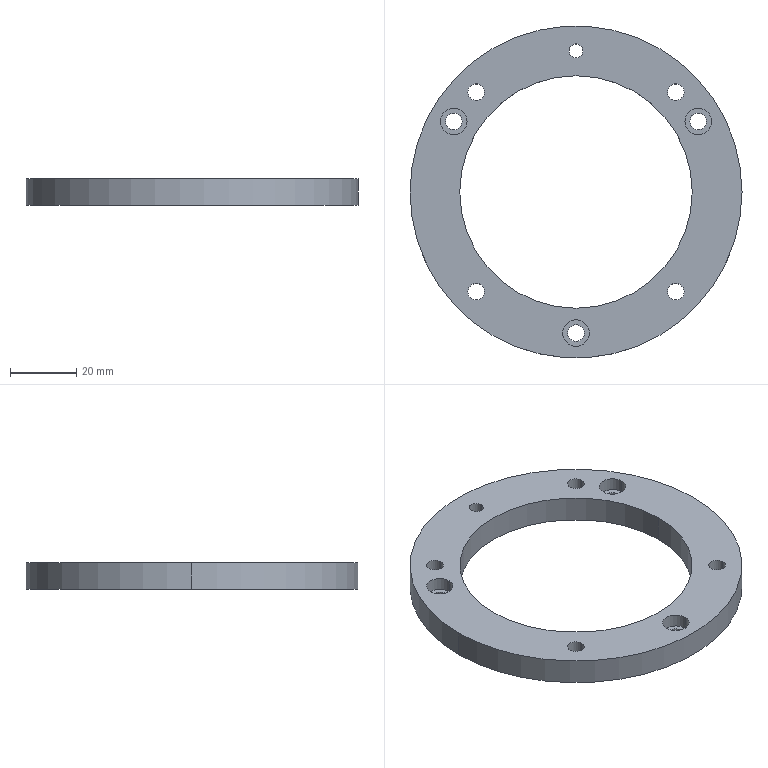Part | SolidWorks | features ICE 5, Extrusion 1 | 1 solid | 31 faces | box 100 x 100 x 8 mm | volume 30466 mm3 | cylinder 26 | plane 5 | commonest cylinder face diameters 5 x14 8 x6 4.2 x2 70 x2 100 x2
STEP:
#1=CARTESIAN_POINT('',(-35.,0.,0.));
#2=VERTEX_POINT('',#1);
#3=CARTESIAN_POINT('',(35.,0.,0.));
#4=VERTEX_POINT('',#3);
#5=CARTESIAN_POINT('',(0.,0.,0.));
#6=DIRECTION('',(0.,0.,1.));
#7=DIRECTION('',(1.,0.,0.));
#8=AXIS2_PLACEMENT_3D('',#5,#6,#7);
#9=CIRCLE('',#8,35.);
#10=EDGE_CURVE('',#2,#4,#9,.T.);
#11=ORIENTED_EDGE('',*,*,#10,.F.);
#12=CARTESIAN_POINT('',(-35.,0.,8.));
#13=VERTEX_POINT('',#12);
#14=CARTESIAN_POINT('',(-35.,0.,-2.));
#15=DIRECTION('',(0.,0.,1.));
#16=VECTOR('',#15,1000.);
#17=LINE('',#14,#16);
#18=EDGE_CURVE('',#2,#13,#17,.T.);
#19=ORIENTED_EDGE('',*,*,#18,.T.);
#20=CARTESIAN_POINT('',(35.,0.,8.));
#21=VERTEX_POINT('',#20);
#22=CARTESIAN_POINT('',(0.,0.,8.));
#23=DIRECTION('',(0.,0.,1.));
#24=DIRECTION('',(1.,0.,0.));
#25=AXIS2_PLACEMENT_3D('',#22,#23,#24);
#26=CIRCLE('',#25,35.);
#27=EDGE_CURVE('',#13,#21,#26,.T.);
#28=ORIENTED_EDGE('',*,*,#27,.T.);
#29=CARTESIAN_POINT('',(35.,0.,-2.));
#30=DIRECTION('',(0.,0.,1.));
#31=VECTOR('',#30,1000.);
#32=LINE('',#29,#31);
#33=EDGE_CURVE('',#4,#21,#32,.T.);
#34=ORIENTED_EDGE('',*,*,#33,.F.);
#35=EDGE_LOOP('',(#11,#19,#28,#34));
#36=FACE_OUTER_BOUND('',#35,.T.);
#37=CARTESIAN_POINT('',(0.,0.,-2.));
#38=DIRECTION('',(0.,0.,1.));
#39=DIRECTION('',(1.,0.,0.));
#40=AXIS2_PLACEMENT_3D('',#37,#38,#39);
#41=CYLINDRICAL_SURFACE('',#40,35.);
#42=ADVANCED_FACE('',(#36),#41,.F.);
#43=CARTESIAN_POINT('',(34.306,21.25,0.));
#44=VERTEX_POINT('',#43);
#45=CARTESIAN_POINT('',(39.306,21.25,0.));
#46=VERTEX_POINT('',#45);
#47=CARTESIAN_POINT('',(36.806,21.25,0.));
#48=DIRECTION('',(0.,0.,1.));
#49=DIRECTION('',(1.,0.,0.));
#50=AXIS2_PLACEMENT_3D('',#47,#48,#49);
#51=CIRCLE('',#50,2.5);
#52=EDGE_CURVE('',#44,#46,#51,.T.);
#53=ORIENTED_EDGE('',*,*,#52,.F.);
#54=CARTESIAN_POINT('',(34.306,21.25,4.));
#55=VERTEX_POINT('',#54);
#56=CARTESIAN_POINT('',(34.306,21.25,0.));
#57=DIRECTION('',(0.,0.,1.));
#58=VECTOR('',#57,1000.);
#59=LINE('',#56,#58);
#60=EDGE_CURVE('',#44,#55,#59,.T.);
#61=ORIENTED_EDGE('',*,*,#60,.T.);
#62=CARTESIAN_POINT('',(39.306,21.25,4.));
#63=VERTEX_POINT('',#62);
#64=CARTESIAN_POINT('',(36.806,21.25,4.));
#65=DIRECTION('',(0.,0.,1.));
#66=DIRECTION('',(1.,0.,0.));
#67=AXIS2_PLACEMENT_3D('',#64,#65,#66);
#68=CIRCLE('',#67,2.5);
#69=EDGE_CURVE('',#55,#63,#68,.T.);
#70=ORIENTED_EDGE('',*,*,#69,.T.);
#71=CARTESIAN_POINT('',(39.306,21.25,0.));
#72=DIRECTION('',(0.,0.,1.));
#73=VECTOR('',#72,1000.);
#74=LINE('',#71,#73);
#75=EDGE_CURVE('',#46,#63,#74,.T.);
#76=ORIENTED_EDGE('',*,*,#75,.F.);
#77=EDGE_LOOP('',(#53,#61,#70,#76));
#78=FACE_OUTER_BOUND('',#77,.T.);
#79=CARTESIAN_POINT('',(36.806,21.25,0.));
#80=DIRECTION('',(0.,0.,1.));
#81=DIRECTION('',(1.,0.,0.));
#82=AXIS2_PLACEMENT_3D('',#79,#80,#81);
#83=CYLINDRICAL_SURFACE('',#82,2.5);
#84=ADVANCED_FACE('',(#78),#83,.F.);
#85=CARTESIAN_POINT('',(-2.5,-42.5,0.));
#86=VERTEX_POINT('',#85);
#87=CARTESIAN_POINT('',(2.5,-42.5,0.));
#88=VERTEX_POINT('',#87);
#89=CARTESIAN_POINT('',(0.,-42.5,0.));
#90=DIRECTION('',(0.,0.,1.));
#91=DIRECTION('',(1.,0.,0.));
#92=AXIS2_PLACEMENT_3D('',#89,#90,#91);
#93=CIRCLE('',#92,2.5);
#94=EDGE_CURVE('',#86,#88,#93,.T.);
#95=ORIENTED_EDGE('',*,*,#94,.F.);
#96=CARTESIAN_POINT('',(-2.5,-42.5,4.));
#97=VERTEX_POINT('',#96);
#98=CARTESIAN_POINT('',(-2.5,-42.5,0.));
#99=DIRECTION('',(0.,0.,1.));
#100=VECTOR('',#99,1000.);
#101=LINE('',#98,#100);
#102=EDGE_CURVE('',#86,#97,#101,.T.);
#103=ORIENTED_EDGE('',*,*,#102,.T.);
#104=CARTESIAN_POINT('',(2.5,-42.5,4.));
#105=VERTEX_POINT('',#104);
#106=CARTESIAN_POINT('',(0.,-42.5,4.));
#107=DIRECTION('',(0.,0.,1.));
#108=DIRECTION('',(1.,0.,0.));
#109=AXIS2_PLACEMENT_3D('',#106,#107,#108);
#110=CIRCLE('',#109,2.5);
#111=EDGE_CURVE('',#97,#105,#110,.T.);
#112=ORIENTED_EDGE('',*,*,#111,.T.);
#113=CARTESIAN_POINT('',(2.5,-42.5,0.));
#114=DIRECTION('',(0.,0.,1.));
#115=VECTOR('',#114,1000.);
#116=LINE('',#113,#115);
#117=EDGE_CURVE('',#88,#105,#116,.T.);
#118=ORIENTED_EDGE('',*,*,#117,.F.);
#119=EDGE_LOOP('',(#95,#103,#112,#118));
#120=FACE_OUTER_BOUND('',#119,.T.);
#121=CARTESIAN_POINT('',(0.,-42.5,0.));
#122=DIRECTION('',(0.,0.,1.));
#123=DIRECTION('',(1.,0.,0.));
#124=AXIS2_PLACEMENT_3D('',#121,#122,#123);
#125=CYLINDRICAL_SURFACE('',#124,2.5);
#126=ADVANCED_FACE('',(#120),#125,.F.);
#127=CARTESIAN_POINT('',(-39.306,21.25,0.));
#128=VERTEX_POINT('',#127);
#129=CARTESIAN_POINT('',(-34.306,21.25,0.));
#130=VERTEX_POINT('',#129);
#131=CARTESIAN_POINT('',(-36.806,21.25,0.));
#132=DIRECTION('',(0.,0.,1.));
#133=DIRECTION('',(1.,0.,0.));
#134=AXIS2_PLACEMENT_3D('',#131,#132,#133);
#135=CIRCLE('',#134,2.5);
#136=EDGE_CURVE('',#128,#130,#135,.T.);
#137=ORIENTED_EDGE('',*,*,#136,.F.);
#138=CARTESIAN_POINT('',(-39.306,21.25,4.));
#139=VERTEX_POINT('',#138);
#140=CARTESIAN_POINT('',(-39.306,21.25,0.));
#141=DIRECTION('',(0.,0.,1.));
#142=VECTOR('',#141,1000.);
#143=LINE('',#140,#142);
#144=EDGE_CURVE('',#128,#139,#143,.T.);
#145=ORIENTED_EDGE('',*,*,#144,.T.);
#146=CARTESIAN_POINT('',(-34.306,21.25,4.));
#147=VERTEX_POINT('',#146);
#148=CARTESIAN_POINT('',(-36.806,21.25,4.));
#149=DIRECTION('',(0.,0.,1.));
#150=DIRECTION('',(1.,0.,0.));
#151=AXIS2_PLACEMENT_3D('',#148,#149,#150);
#152=CIRCLE('',#151,2.5);
#153=EDGE_CURVE('',#139,#147,#152,.T.);
#154=ORIENTED_EDGE('',*,*,#153,.T.);
#155=CARTESIAN_POINT('',(-34.306,21.25,0.));
#156=DIRECTION('',(0.,0.,1.));
#157=VECTOR('',#156,1000.);
#158=LINE('',#155,#157);
#159=EDGE_CURVE('',#130,#147,#158,.T.);
#160=ORIENTED_EDGE('',*,*,#159,.F.);
#161=EDGE_LOOP('',(#137,#145,#154,#160));
#162=FACE_OUTER_BOUND('',#161,.T.);
#163=CARTESIAN_POINT('',(-36.806,21.25,0.));
#164=DIRECTION('',(0.,0.,1.));
#165=DIRECTION('',(1.,0.,0.));
#166=AXIS2_PLACEMENT_3D('',#163,#164,#165);
#167=CYLINDRICAL_SURFACE('',#166,2.5);
#168=ADVANCED_FACE('',(#162),#167,.F.);
#169=CARTESIAN_POINT('',(32.806,21.25,4.));
#170=VERTEX_POINT('',#169);
#171=CARTESIAN_POINT('',(40.806,21.25,4.));
#172=VERTEX_POINT('',#171);
#173=CARTESIAN_POINT('',(36.806,21.25,4.));
#174=DIRECTION('',(0.,0.,1.));
#175=DIRECTION('',(1.,0.,0.));
#176=AXIS2_PLACEMENT_3D('',#173,#174,#175);
#177=CIRCLE('',#176,4.);
#178=EDGE_CURVE('',#170,#172,#177,.T.);
#179=ORIENTED_EDGE('',*,*,#178,.F.);
#180=CARTESIAN_POINT('',(32.806,21.25,8.));
#181=VERTEX_POINT('',#180);
#182=CARTESIAN_POINT('',(32.806,21.25,4.));
#183=DIRECTION('',(0.,0.,1.));
#184=VECTOR('',#183,1000.);
#185=LINE('',#182,#184);
#186=EDGE_CURVE('',#170,#181,#185,.T.);
#187=ORIENTED_EDGE('',*,*,#186,.T.);
#188=CARTESIAN_POINT('',(40.806,21.25,8.));
#189=VERTEX_POINT('',#188);
#190=CARTESIAN_POINT('',(36.806,21.25,8.));
#191=DIRECTION('',(0.,0.,1.));
#192=DIRECTION('',(1.,0.,0.));
#193=AXIS2_PLACEMENT_3D('',#190,#191,#192);
#194=CIRCLE('',#193,4.);
#195=EDGE_CURVE('',#181,#189,#194,.T.);
#196=ORIENTED_EDGE('',*,*,#195,.T.);
#197=CARTESIAN_POINT('',(40.806,21.25,4.));
#198=DIRECTION('',(0.,0.,1.));
#199=VECTOR('',#198,1000.);
#200=LINE('',#197,#199);
#201=EDGE_CURVE('',#172,#189,#200,.T.);
#202=ORIENTED_EDGE('',*,*,#201,.F.);
#203=EDGE_LOOP('',(#179,#187,#196,#202));
#204=FACE_OUTER_BOUND('',#203,.T.);
#205=CARTESIAN_POINT('',(36.806,21.25,4.));
#206=DIRECTION('',(0.,0.,1.));
#207=DIRECTION('',(1.,0.,0.));
#208=AXIS2_PLACEMENT_3D('',#205,#206,#207);
#209=CYLINDRICAL_SURFACE('',#208,4.);
#210=ADVANCED_FACE('',(#204),#209,.F.);
#211=CARTESIAN_POINT('',(-40.806,21.25,4.));
#212=VERTEX_POINT('',#211);
#213=CARTESIAN_POINT('',(-32.806,21.25,4.));
#214=VERTEX_POINT('',#213);
#215=CARTESIAN_POINT('',(-36.806,21.25,4.));
#216=DIRECTION('',(0.,0.,1.));
#217=DIRECTION('',(1.,0.,0.));
#218=AXIS2_PLACEMENT_3D('',#215,#216,#217);
#219=CIRCLE('',#218,4.);
#220=EDGE_CURVE('',#212,#214,#219,.T.);
#221=ORIENTED_EDGE('',*,*,#220,.F.);
#222=CARTESIAN_POINT('',(-40.806,21.25,8.));
#223=VERTEX_POINT('',#222);
#224=CARTESIAN_POINT('',(-40.806,21.25,4.));
#225=DIRECTION('',(0.,0.,1.));
#226=VECTOR('',#225,1000.);
#227=LINE('',#224,#226);
#228=EDGE_CURVE('',#212,#223,#227,.T.);
#229=ORIENTED_EDGE('',*,*,#228,.T.);
#230=CARTESIAN_POINT('',(-32.806,21.25,8.));
#231=VERTEX_POINT('',#230);
#232=CARTESIAN_POINT('',(-36.806,21.25,8.));
#233=DIRECTION('',(0.,0.,1.));
#234=DIRECTION('',(1.,0.,0.));
#235=AXIS2_PLACEMENT_3D('',#232,#233,#234);
#236=CIRCLE('',#235,4.);
#237=EDGE_CURVE('',#223,#231,#236,.T.);
#238=ORIENTED_EDGE('',*,*,#237,.T.);
#239=CARTESIAN_POINT('',(-32.806,21.25,4.));
#240=DIRECTION('',(0.,0.,1.));
#241=VECTOR('',#240,1000.);
#242=LINE('',#239,#241);
#243=EDGE_CURVE('',#214,#231,#242,.T.);
#244=ORIENTED_EDGE('',*,*,#243,.F.);
#245=EDGE_LOOP('',(#221,#229,#238,#244));
#246=FACE_OUTER_BOUND('',#245,.T.);
#247=CARTESIAN_POINT('',(-36.806,21.25,4.));
#248=DIRECTION('',(0.,0.,1.));
#249=DIRECTION('',(1.,0.,0.));
#250=AXIS2_PLACEMENT_3D('',#247,#248,#249);
#251=CYLINDRICAL_SURFACE('',#250,4.);
#252=ADVANCED_FACE('',(#246),#251,.F.);
#253=CARTESIAN_POINT('',(-4.,-42.5,4.));
#254=VERTEX_POINT('',#253);
#255=CARTESIAN_POINT('',(4.,-42.5,4.));
#256=VERTEX_POINT('',#255);
#257=CARTESIAN_POINT('',(0.,-42.5,4.));
#258=DIRECTION('',(0.,0.,1.));
#259=DIRECTION('',(1.,0.,0.));
#260=AXIS2_PLACEMENT_3D('',#257,#258,#259);
#261=CIRCLE('',#260,4.);
#262=EDGE_CURVE('',#254,#256,#261,.T.);
#263=ORIENTED_EDGE('',*,*,#262,.F.);
#264=CARTESIAN_POINT('',(-4.,-42.5,8.));
#265=VERTEX_POINT('',#264);
#266=CARTESIAN_POINT('',(-4.,-42.5,4.));
#267=DIRECTION('',(0.,0.,1.));
#268=VECTOR('',#267,1000.);
#269=LINE('',#266,#268);
#270=EDGE_CURVE('',#254,#265,#269,.T.);
#271=ORIENTED_EDGE('',*,*,#270,.T.);
#272=CARTESIAN_POINT('',(4.,-42.5,8.));
#273=VERTEX_POINT('',#272);
#274=CARTESIAN_POINT('',(0.,-42.5,8.));
#275=DIRECTION('',(0.,0.,1.));
#276=DIRECTION('',(1.,0.,0.));
#277=AXIS2_PLACEMENT_3D('',#274,#275,#276);
#278=CIRCLE('',#277,4.);
#279=EDGE_CURVE('',#265,#273,#278,.T.);
#280=ORIENTED_EDGE('',*,*,#279,.T.);
#281=CARTESIAN_POINT('',(4.,-42.5,4.));
#282=DIRECTION('',(0.,0.,1.));
#283=VECTOR('',#282,1000.);
#284=LINE('',#281,#283);
#285=EDGE_CURVE('',#256,#273,#284,.T.);
#286=ORIENTED_EDGE('',*,*,#285,.F.);
#287=EDGE_LOOP('',(#263,#271,#280,#286));
#288=FACE_OUTER_BOUND('',#287,.T.);
#289=CARTESIAN_POINT('',(0.,-42.5,4.));
#290=DIRECTION('',(0.,0.,1.));
#291=DIRECTION('',(1.,0.,0.));
#292=AXIS2_PLACEMENT_3D('',#289,#290,#291);
#293=CYLINDRICAL_SURFACE('',#292,4.);
#294=ADVANCED_FACE('',(#288),#293,.F.);
#295=CARTESIAN_POINT('',(-2.1,42.5,0.));
#296=VERTEX_POINT('',#295);
#297=CARTESIAN_POINT('',(2.1,42.5,0.));
#298=VERTEX_POINT('',#297);
#299=CARTESIAN_POINT('',(0.,42.5,0.));
#300=DIRECTION('',(0.,0.,1.));
#301=DIRECTION('',(1.,0.,0.));
#302=AXIS2_PLACEMENT_3D('',#299,#300,#301);
#303=CIRCLE('',#302,2.1);
#304=EDGE_CURVE('',#296,#298,#303,.T.);
#305=ORIENTED_EDGE('',*,*,#304,.F.);
#306=CARTESIAN_POINT('',(-2.1,42.5,8.));
#307=VERTEX_POINT('',#306);
#308=CARTESIAN_POINT('',(-2.1,42.5,0.));
#309=DIRECTION('',(0.,0.,1.));
#310=VECTOR('',#309,1000.);
#311=LINE('',#308,#310);
#312=EDGE_CURVE('',#296,#307,#311,.T.);
#313=ORIENTED_EDGE('',*,*,#312,.T.);
#314=CARTESIAN_POINT('',(2.1,42.5,8.));
#315=VERTEX_POINT('',#314);
#316=CARTESIAN_POINT('',(0.,42.5,8.));
#317=DIRECTION('',(0.,0.,1.));
#318=DIRECTION('',(1.,0.,0.));
#319=AXIS2_PLACEMENT_3D('',#316,#317,#318);
#320=CIRCLE('',#319,2.1);
#321=EDGE_CURVE('',#307,#315,#320,.T.);
#322=ORIENTED_EDGE('',*,*,#321,.T.);
#323=CARTESIAN_POINT('',(2.1,42.5,0.));
#324=DIRECTION('',(0.,0.,1.));
#325=VECTOR('',#324,1000.);
#326=LINE('',#323,#325);
#327=EDGE_CURVE('',#298,#315,#326,.T.);
#328=ORIENTED_EDGE('',*,*,#327,.F.);
#329=EDGE_LOOP('',(#305,#313,#322,#328));
#330=FACE_OUTER_BOUND('',#329,.T.);
#331=CARTESIAN_POINT('',(0.,42.5,0.));
#332=DIRECTION('',(0.,0.,1.));
#333=DIRECTION('',(1.,0.,0.));
#334=AXIS2_PLACEMENT_3D('',#331,#332,#333);
#335=CYLINDRICAL_SURFACE('',#334,2.1);
#336=ADVANCED_FACE('',(#330),#335,.F.);
#337=CARTESIAN_POINT('',(27.554,-30.05,0.));
#338=VERTEX_POINT('',#337);
#339=CARTESIAN_POINT('',(32.554,-30.05,0.));
#340=VERTEX_POINT('',#339);
#341=CARTESIAN_POINT('',(30.054,-30.05,0.));
#342=DIRECTION('',(0.,0.,1.));
#343=DIRECTION('',(1.,0.,0.));
#344=AXIS2_PLACEMENT_3D('',#341,#342,#343);
#345=CIRCLE('',#344,2.5);
#346=EDGE_CURVE('',#338,#340,#345,.T.);
#347=ORIENTED_EDGE('',*,*,#346,.F.);
#348=CARTESIAN_POINT('',(27.554,-30.05,8.));
#349=VERTEX_POINT('',#348);
#350=CARTESIAN_POINT('',(27.554,-30.05,0.));
#351=DIRECTION('',(0.,0.,1.));
#352=VECTOR('',#351,1000.);
#353=LINE('',#350,#352);
#354=EDGE_CURVE('',#338,#349,#353,.T.);
#355=ORIENTED_EDGE('',*,*,#354,.T.);
#356=CARTESIAN_POINT('',(32.554,-30.05,8.));
#357=VERTEX_POINT('',#356);
#358=CARTESIAN_POINT('',(30.054,-30.05,8.));
#359=DIRECTION('',(0.,0.,1.));
#360=DIRECTION('',(1.,0.,0.));
#361=AXIS2_PLACEMENT_3D('',#358,#359,#360);
#362=CIRCLE('',#361,2.5);
#363=EDGE_CURVE('',#349,#357,#362,.T.);
#364=ORIENTED_EDGE('',*,*,#363,.T.);
#365=CARTESIAN_POINT('',(32.554,-30.05,0.));
#366=DIRECTION('',(0.,0.,1.));
#367=VECTOR('',#366,1000.);
#368=LINE('',#365,#367);
#369=EDGE_CURVE('',#340,#357,#368,.T.);
#370=ORIENTED_EDGE('',*,*,#369,.F.);
#371=EDGE_LOOP('',(#347,#355,#364,#370));
#372=FACE_OUTER_BOUND('',#371,.T.);
#373=CARTESIAN_POINT('',(30.054,-30.05,0.));
#374=DIRECTION('',(0.,0.,1.));
#375=DIRECTION('',(1.,0.,0.));
#376=AXIS2_PLACEMENT_3D('',#373,#374,#375);
#377=CYLINDRICAL_SURFACE('',#376,2.5);
#378=ADVANCED_FACE('',(#372),#377,.F.);
#379=CARTESIAN_POINT('',(-32.554,-30.05,0.));
#380=VERTEX_POINT('',#379);
#381=CARTESIAN_POINT('',(-27.554,-30.05,0.));
#382=VERTEX_POINT('',#381);
#383=CARTESIAN_POINT('',(-30.054,-30.05,0.));
#384=DIRECTION('',(0.,0.,1.));
#385=DIRECTION('',(1.,0.,0.));
#386=AXIS2_PLACEMENT_3D('',#383,#384,#385);
#387=CIRCLE('',#386,2.5);
#388=EDGE_CURVE('',#380,#382,#387,.T.);
#389=ORIENTED_EDGE('',*,*,#388,.F.);
#390=CARTESIAN_POINT('',(-32.554,-30.05,8.));
#391=VERTEX_POINT('',#390);
#392=CARTESIAN_POINT('',(-32.554,-30.05,0.));
#393=DIRECTION('',(0.,0.,1.));
#394=VECTOR('',#393,1000.);
#395=LINE('',#392,#394);
#396=EDGE_CURVE('',#380,#391,#395,.T.);
#397=ORIENTED_EDGE('',*,*,#396,.T.);
#398=CARTESIAN_POINT('',(-27.554,-30.05,8.));
#399=VERTEX_POINT('',#398);
#400=CARTESIAN_POINT('',(-30.054,-30.05,8.));
#401=DIRECTION('',(0.,0.,1.));
#402=DIRECTION('',(1.,0.,0.));
#403=AXIS2_PLACEMENT_3D('',#400,#401,#402);
#404=CIRCLE('',#403,2.5);
#405=EDGE_CURVE('',#391,#399,#404,.T.);
#406=ORIENTED_EDGE('',*,*,#405,.T.);
#407=CARTESIAN_POINT('',(-27.554,-30.05,0.));
#408=DIRECTION('',(0.,0.,1.));
#409=VECTOR('',#408,1000.);
#410=LINE('',#407,#409);
#411=EDGE_CURVE('',#382,#399,#410,.T.);
#412=ORIENTED_EDGE('',*,*,#411,.F.);
#413=EDGE_LOOP('',(#389,#397,#406,#412));
#414=FACE_OUTER_BOUND('',#413,.T.);
#415=CARTESIAN_POINT('',(-30.054,-30.05,0.));
#416=DIRECTION('',(0.,0.,1.));
#417=DIRECTION('',(1.,0.,0.));
#418=AXIS2_PLACEMENT_3D('',#415,#416,#417);
#419=CYLINDRICAL_SURFACE('',#418,2.5);
#420=ADVANCED_FACE('',(#414),#419,.F.);
#421=CARTESIAN_POINT('',(27.554,30.05,0.));
#422=VERTEX_POINT('',#421);
#423=CARTESIAN_POINT('',(32.554,30.05,0.));
#424=VERTEX_POINT('',#423);
#425=CARTESIAN_POINT('',(30.054,30.05,0.));
#426=DIRECTION('',(0.,0.,1.));
#427=DIRECTION('',(1.,0.,0.));
#428=AXIS2_PLACEMENT_3D('',#425,#426,#427);
#429=CIRCLE('',#428,2.5);
#430=EDGE_CURVE('',#422,#424,#429,.T.);
#431=ORIENTED_EDGE('',*,*,#430,.F.);
#432=CARTESIAN_POINT('',(27.554,30.05,8.));
#433=VERTEX_POINT('',#432);
#434=CARTESIAN_POINT('',(27.554,30.05,0.));
#435=DIRECTION('',(0.,0.,1.));
#436=VECTOR('',#435,1000.);
#437=LINE('',#434,#436);
#438=EDGE_CURVE('',#422,#433,#437,.T.);
#439=ORIENTED_EDGE('',*,*,#438,.T.);
#440=CARTESIAN_POINT('',(32.554,30.05,8.));
#441=VERTEX_POINT('',#440);
#442=CARTESIAN_POINT('',(30.054,30.05,8.));
#443=DIRECTION('',(0.,0.,1.));
#444=DIRECTION('',(1.,0.,0.));
#445=AXIS2_PLACEMENT_3D('',#442,#443,#444);
#446=CIRCLE('',#445,2.5);
#447=EDGE_CURVE('',#433,#441,#446,.T.);
#448=ORIENTED_EDGE('',*,*,#447,.T.);
#449=CARTESIAN_POINT('',(32.554,30.05,0.));
#450=DIRECTION('',(0.,0.,1.));
#451=VECTOR('',#450,1000.);
#452=LINE('',#449,#451);
#453=EDGE_CURVE('',#424,#441,#452,.T.);
#454=ORIENTED_EDGE('',*,*,#453,.F.);
#455=EDGE_LOOP('',(#431,#439,#448,#454));
#456=FACE_OUTER_BOUND('',#455,.T.);
#457=CARTESIAN_POINT('',(30.054,30.05,0.));
#458=DIRECTION('',(0.,0.,1.));
#459=DIRECTION('',(1.,0.,0.));
#460=AXIS2_PLACEMENT_3D('',#457,#458,#459);
#461=CYLINDRICAL_SURFACE('',#460,2.5);
#462=ADVANCED_FACE('',(#456),#461,.F.);
#463=CARTESIAN_POINT('',(-32.554,30.05,0.));
#464=VERTEX_POINT('',#463);
#465=CARTESIAN_POINT('',(-27.554,30.05,0.));
#466=VERTEX_POINT('',#465);
#467=CARTESIAN_POINT('',(-30.054,30.05,0.));
#468=DIRECTION('',(0.,0.,1.));
#469=DIRECTION('',(1.,0.,0.));
#470=AXIS2_PLACEMENT_3D('',#467,#468,#469);
#471=CIRCLE('',#470,2.5);
#472=EDGE_CURVE('',#464,#466,#471,.T.);
#473=ORIENTED_EDGE('',*,*,#472,.F.);
#474=CARTESIAN_POINT('',(-32.554,30.05,8.));
#475=VERTEX_POINT('',#474);
#476=CARTESIAN_POINT('',(-32.554,30.05,0.));
#477=DIRECTION('',(0.,0.,1.));
#478=VECTOR('',#477,1000.);
#479=LINE('',#476,#478);
#480=EDGE_CURVE('',#464,#475,#479,.T.);
#481=ORIENTED_EDGE('',*,*,#480,.T.);
#482=CARTESIAN_POINT('',(-27.554,30.05,8.));
#483=VERTEX_POINT('',#482);
#484=CARTESIAN_POINT('',(-30.054,30.05,8.));
#485=DIRECTION('',(0.,0.,1.));
#486=DIRECTION('',(1.,0.,0.));
#487=AXIS2_PLACEMENT_3D('',#484,#485,#486);
#488=CIRCLE('',#487,2.5);
#489=EDGE_CURVE('',#475,#483,#488,.T.);
#490=ORIENTED_EDGE('',*,*,#489,.T.);
#491=CARTESIAN_POINT('',(-27.554,30.05,0.));
#492=DIRECTION('',(0.,0.,1.));
#493=VECTOR('',#492,1000.);
#494=LINE('',#491,#493);
#495=EDGE_CURVE('',#466,#483,#494,.T.);
#496=ORIENTED_EDGE('',*,*,#495,.F.);
#497=EDGE_LOOP('',(#473,#481,#490,#496));
#498=FACE_OUTER_BOUND('',#497,.T.);
#499=CARTESIAN_POINT('',(-30.054,30.05,0.));
#500=DIRECTION('',(0.,0.,1.));
#501=DIRECTION('',(1.,0.,0.));
#502=AXIS2_PLACEMENT_3D('',#499,#500,#501);
#503=CYLINDRICAL_SURFACE('',#502,2.5);
#504=ADVANCED_FACE('',(#498),#503,.F.);
#505=CARTESIAN_POINT('',(50.,0.,8.));
#506=VERTEX_POINT('',#505);
#507=CARTESIAN_POINT('',(-50.,0.,8.));
#508=VERTEX_POINT('',#507);
#509=CARTESIAN_POINT('',(0.,0.,8.));
#510=DIRECTION('',(0.,0.,1.));
#511=DIRECTION('',(1.,0.,0.));
#512=AXIS2_PLACEMENT_3D('',#509,#510,#511);
#513=CIRCLE('',#512,50.);
#514=EDGE_CURVE('',#506,#508,#513,.T.);
#515=ORIENTED_EDGE('',*,*,#514,.F.);
#516=CARTESIAN_POINT('',(50.,0.,0.));
#517=VERTEX_POINT('',#516);
#518=CARTESIAN_POINT('',(50.,0.,8.));
#519=DIRECTION('',(0.,0.,-1.));
#520=VECTOR('',#519,1000.);
#521=LINE('',#518,#520);
#522=EDGE_CURVE('',#506,#517,#521,.T.);
#523=ORIENTED_EDGE('',*,*,#522,.T.);
#524=CARTESIAN_POINT('',(-50.,0.,0.));
#525=VERTEX_POINT('',#524);
#526=CARTESIAN_POINT('',(0.,0.,0.));
#527=DIRECTION('',(0.,0.,1.));
#528=DIRECTION('',(1.,0.,0.));
#529=AXIS2_PLACEMENT_3D('',#526,#527,#528);
#530=CIRCLE('',#529,50.);
#531=EDGE_CURVE('',#517,#525,#530,.T.);
#532=ORIENTED_EDGE('',*,*,#531,.T.);
#533=CARTESIAN_POINT('',(-50.,0.,8.));
#534=DIRECTION('',(0.,0.,-1.));
#535=VECTOR('',#534,1000.);
#536=LINE('',#533,#535);
#537=EDGE_CURVE('',#508,#525,#536,.T.);
#538=ORIENTED_EDGE('',*,*,#537,.F.);
#539=EDGE_LOOP('',(#515,#523,#532,#538));
#540=FACE_OUTER_BOUND('',#539,.T.);
#541=CARTESIAN_POINT('',(0.,0.,8.));
#542=DIRECTION('',(0.,0.,-1.));
#543=DIRECTION('',(-1.,0.,0.));
#544=AXIS2_PLACEMENT_3D('',#541,#542,#543);
#545=CYLINDRICAL_SURFACE('',#544,50.);
#546=ADVANCED_FACE('',(#540),#545,.T.);
#547=ORIENTED_EDGE('',*,*,#522,.F.);
#548=CARTESIAN_POINT('',(0.,0.,8.));
#549=DIRECTION('',(0.,0.,1.));
#550=DIRECTION('',(1.,0.,0.));
#551=AXIS2_PLACEMENT_3D('',#548,#549,#550);
#552=CIRCLE('',#551,50.);
#553=EDGE_CURVE('',#508,#506,#552,.T.);
#554=ORIENTED_EDGE('',*,*,#553,.F.);
#555=ORIENTED_EDGE('',*,*,#537,.T.);
#556=CARTESIAN_POINT('',(0.,0.,0.));
#557=DIRECTION('',(0.,0.,1.));
#558=DIRECTION('',(1.,0.,0.));
#559=AXIS2_PLACEMENT_3D('',#556,#557,#558);
#560=CIRCLE('',#559,50.);
#561=EDGE_CURVE('',#525,#517,#560,.T.);
#562=ORIENTED_EDGE('',*,*,#561,.T.);
#563=EDGE_LOOP('',(#547,#554,#555,#562));
#564=FACE_OUTER_BOUND('',#563,.T.);
#565=CARTESIAN_POINT('',(0.,0.,8.));
#566=DIRECTION('',(0.,0.,-1.));
#567=DIRECTION('',(-1.,0.,0.));
#568=AXIS2_PLACEMENT_3D('',#565,#566,#567);
#569=CYLINDRICAL_SURFACE('',#568,50.);
#570=ADVANCED_FACE('',(#564),#569,.T.);
#571=CARTESIAN_POINT('',(0.,0.,8.));
#572=DIRECTION('',(0.,0.,1.));
#573=DIRECTION('',(1.,0.,0.));
#574=AXIS2_PLACEMENT_3D('',#571,#572,#573);
#575=CIRCLE('',#574,35.);
#576=EDGE_CURVE('',#21,#13,#575,.T.);
#577=ORIENTED_EDGE('',*,*,#576,.F.);
#578=ORIENTED_EDGE('',*,*,#27,.F.);
#579=EDGE_LOOP('',(#577,#578));
#580=FACE_BOUND('',#579,.T.);
#581=CARTESIAN_POINT('',(36.806,21.25,8.));
#582=DIRECTION('',(0.,0.,1.));
#583=DIRECTION('',(1.,0.,0.));
#584=AXIS2_PLACEMENT_3D('',#581,#582,#583);
#585=CIRCLE('',#584,4.);
#586=EDGE_CURVE('',#189,#181,#585,.T.);
#587=ORIENTED_EDGE('',*,*,#586,.F.);
#588=ORIENTED_EDGE('',*,*,#195,.F.);
#589=EDGE_LOOP('',(#587,#588));
#590=FACE_BOUND('',#589,.T.);
#591=CARTESIAN_POINT('',(-36.806,21.25,8.));
#592=DIRECTION('',(0.,0.,1.));
#593=DIRECTION('',(1.,0.,0.));
#594=AXIS2_PLACEMENT_3D('',#591,#592,#593);
#595=CIRCLE('',#594,4.);
#596=EDGE_CURVE('',#231,#223,#595,.T.);
#597=ORIENTED_EDGE('',*,*,#596,.F.);
#598=ORIENTED_EDGE('',*,*,#237,.F.);
#599=EDGE_LOOP('',(#597,#598));
#600=FACE_BOUND('',#599,.T.);
#601=CARTESIAN_POINT('',(0.,-42.5,8.));
#602=DIRECTION('',(0.,0.,1.));
#603=DIRECTION('',(1.,0.,0.));
#604=AXIS2_PLACEMENT_3D('',#601,#602,#603);
#605=CIRCLE('',#604,4.);
#606=EDGE_CURVE('',#273,#265,#605,.T.);
#607=ORIENTED_EDGE('',*,*,#606,.F.);
#608=ORIENTED_EDGE('',*,*,#279,.F.);
#609=EDGE_LOOP('',(#607,#608));
#610=FACE_BOUND('',#609,.T.);
#611=CARTESIAN_POINT('',(0.,42.5,8.));
#612=DIRECTION('',(0.,0.,1.));
#613=DIRECTION('',(1.,0.,0.));
#614=AXIS2_PLACEMENT_3D('',#611,#612,#613);
#615=CIRCLE('',#614,2.1);
#616=EDGE_CURVE('',#315,#307,#615,.T.);
#617=ORIENTED_EDGE('',*,*,#616,.F.);
#618=ORIENTED_EDGE('',*,*,#321,.F.);
#619=EDGE_LOOP('',(#617,#618));
#620=FACE_BOUND('',#619,.T.);
#621=CARTESIAN_POINT('',(30.054,-30.05,8.));
#622=DIRECTION('',(0.,0.,1.));
#623=DIRECTION('',(1.,0.,0.));
#624=AXIS2_PLACEMENT_3D('',#621,#622,#623);
#625=CIRCLE('',#624,2.5);
#626=EDGE_CURVE('',#357,#349,#625,.T.);
#627=ORIENTED_EDGE('',*,*,#626,.F.);
#628=ORIENTED_EDGE('',*,*,#363,.F.);
#629=EDGE_LOOP('',(#627,#628));
#630=FACE_BOUND('',#629,.T.);
#631=CARTESIAN_POINT('',(-30.054,-30.05,8.));
#632=DIRECTION('',(0.,0.,1.));
#633=DIRECTION('',(1.,0.,0.));
#634=AXIS2_PLACEMENT_3D('',#631,#632,#633);
#635=CIRCLE('',#634,2.5);
#636=EDGE_CURVE('',#399,#391,#635,.T.);
#637=ORIENTED_EDGE('',*,*,#636,.F.);
#638=ORIENTED_EDGE('',*,*,#405,.F.);
#639=EDGE_LOOP('',(#637,#638));
#640=FACE_BOUND('',#639,.T.);
#641=CARTESIAN_POINT('',(30.054,30.05,8.));
#642=DIRECTION('',(0.,0.,1.));
#643=DIRECTION('',(1.,0.,0.));
#644=AXIS2_PLACEMENT_3D('',#641,#642,#643);
#645=CIRCLE('',#644,2.5);
#646=EDGE_CURVE('',#441,#433,#645,.T.);
#647=ORIENTED_EDGE('',*,*,#646,.F.);
#648=ORIENTED_EDGE('',*,*,#447,.F.);
#649=EDGE_LOOP('',(#647,#648));
#650=FACE_BOUND('',#649,.T.);
#651=CARTESIAN_POINT('',(-30.054,30.05,8.));
#652=DIRECTION('',(0.,0.,1.));
#653=DIRECTION('',(1.,0.,0.));
#654=AXIS2_PLACEMENT_3D('',#651,#652,#653);
#655=CIRCLE('',#654,2.5);
#656=EDGE_CURVE('',#483,#475,#655,.T.);
#657=ORIENTED_EDGE('',*,*,#656,.F.);
#658=ORIENTED_EDGE('',*,*,#489,.F.);
#659=EDGE_LOOP('',(#657,#658));
#660=FACE_BOUND('',#659,.T.);
#661=ORIENTED_EDGE('',*,*,#553,.T.);
#662=ORIENTED_EDGE('',*,*,#514,.T.);
#663=EDGE_LOOP('',(#661,#662));
#664=FACE_OUTER_BOUND('',#663,.T.);
#665=CARTESIAN_POINT('',(0.,0.,8.));
#666=DIRECTION('',(0.,0.,1.));
#667=DIRECTION('',(1.,0.,0.));
#668=AXIS2_PLACEMENT_3D('',#665,#666,#667);
#669=PLANE('',#668);
#670=ADVANCED_FACE('',(#580,#590,#600,#610,#620,#630,#640,#650,#660,#664),#669,.T.);
#671=CARTESIAN_POINT('',(0.,0.,0.));
#672=DIRECTION('',(0.,0.,1.));
#673=DIRECTION('',(1.,0.,0.));
#674=AXIS2_PLACEMENT_3D('',#671,#672,#673);
#675=CIRCLE('',#674,35.);
#676=EDGE_CURVE('',#4,#2,#675,.T.);
#677=ORIENTED_EDGE('',*,*,#676,.T.);
#678=ORIENTED_EDGE('',*,*,#10,.T.);
#679=EDGE_LOOP('',(#677,#678));
#680=FACE_BOUND('',#679,.T.);
#681=CARTESIAN_POINT('',(36.806,21.25,0.));
#682=DIRECTION('',(0.,0.,1.));
#683=DIRECTION('',(1.,0.,0.));
#684=AXIS2_PLACEMENT_3D('',#681,#682,#683);
#685=CIRCLE('',#684,2.5);
#686=EDGE_CURVE('',#46,#44,#685,.T.);
#687=ORIENTED_EDGE('',*,*,#686,.T.);
#688=ORIENTED_EDGE('',*,*,#52,.T.);
#689=EDGE_LOOP('',(#687,#688));
#690=FACE_BOUND('',#689,.T.);
#691=CARTESIAN_POINT('',(0.,-42.5,0.));
#692=DIRECTION('',(0.,0.,1.));
#693=DIRECTION('',(1.,0.,0.));
#694=AXIS2_PLACEMENT_3D('',#691,#692,#693);
#695=CIRCLE('',#694,2.5);
#696=EDGE_CURVE('',#88,#86,#695,.T.);
#697=ORIENTED_EDGE('',*,*,#696,.T.);
#698=ORIENTED_EDGE('',*,*,#94,.T.);
#699=EDGE_LOOP('',(#697,#698));
#700=FACE_BOUND('',#699,.T.);
#701=CARTESIAN_POINT('',(-36.806,21.25,0.));
#702=DIRECTION('',(0.,0.,1.));
#703=DIRECTION('',(1.,0.,0.));
#704=AXIS2_PLACEMENT_3D('',#701,#702,#703);
#705=CIRCLE('',#704,2.5);
#706=EDGE_CURVE('',#130,#128,#705,.T.);
#707=ORIENTED_EDGE('',*,*,#706,.T.);
#708=ORIENTED_EDGE('',*,*,#136,.T.);
#709=EDGE_LOOP('',(#707,#708));
#710=FACE_BOUND('',#709,.T.);
#711=CARTESIAN_POINT('',(0.,42.5,0.));
#712=DIRECTION('',(0.,0.,1.));
#713=DIRECTION('',(1.,0.,0.));
#714=AXIS2_PLACEMENT_3D('',#711,#712,#713);
#715=CIRCLE('',#714,2.1);
#716=EDGE_CURVE('',#298,#296,#715,.T.);
#717=ORIENTED_EDGE('',*,*,#716,.T.);
#718=ORIENTED_EDGE('',*,*,#304,.T.);
#719=EDGE_LOOP('',(#717,#718));
#720=FACE_BOUND('',#719,.T.);
#721=CARTESIAN_POINT('',(30.054,-30.05,0.));
#722=DIRECTION('',(0.,0.,1.));
#723=DIRECTION('',(1.,0.,0.));
#724=AXIS2_PLACEMENT_3D('',#721,#722,#723);
#725=CIRCLE('',#724,2.5);
#726=EDGE_CURVE('',#340,#338,#725,.T.);
#727=ORIENTED_EDGE('',*,*,#726,.T.);
#728=ORIENTED_EDGE('',*,*,#346,.T.);
#729=EDGE_LOOP('',(#727,#728));
#730=FACE_BOUND('',#729,.T.);
#731=CARTESIAN_POINT('',(-30.054,-30.05,0.));
#732=DIRECTION('',(0.,0.,1.));
#733=DIRECTION('',(1.,0.,0.));
#734=AXIS2_PLACEMENT_3D('',#731,#732,#733);
#735=CIRCLE('',#734,2.5);
#736=EDGE_CURVE('',#382,#380,#735,.T.);
#737=ORIENTED_EDGE('',*,*,#736,.T.);
#738=ORIENTED_EDGE('',*,*,#388,.T.);
#739=EDGE_LOOP('',(#737,#738));
#740=FACE_BOUND('',#739,.T.);
#741=CARTESIAN_POINT('',(30.054,30.05,0.));
#742=DIRECTION('',(0.,0.,1.));
#743=DIRECTION('',(1.,0.,0.));
#744=AXIS2_PLACEMENT_3D('',#741,#742,#743);
#745=CIRCLE('',#744,2.5);
#746=EDGE_CURVE('',#424,#422,#745,.T.);
#747=ORIENTED_EDGE('',*,*,#746,.T.);
#748=ORIENTED_EDGE('',*,*,#430,.T.);
#749=EDGE_LOOP('',(#747,#748));
#750=FACE_BOUND('',#749,.T.);
#751=CARTESIAN_POINT('',(-30.054,30.05,0.));
#752=DIRECTION('',(0.,0.,1.));
#753=DIRECTION('',(1.,0.,0.));
#754=AXIS2_PLACEMENT_3D('',#751,#752,#753);
#755=CIRCLE('',#754,2.5);
#756=EDGE_CURVE('',#466,#464,#755,.T.);
#757=ORIENTED_EDGE('',*,*,#756,.T.);
#758=ORIENTED_EDGE('',*,*,#472,.T.);
#759=EDGE_LOOP('',(#757,#758));
#760=FACE_BOUND('',#759,.T.);
#761=ORIENTED_EDGE('',*,*,#561,.F.);
#762=ORIENTED_EDGE('',*,*,#531,.F.);
#763=EDGE_LOOP('',(#761,#762));
#764=FACE_OUTER_BOUND('',#763,.T.);
#765=CARTESIAN_POINT('',(0.,0.,0.));
#766=DIRECTION('',(0.,0.,1.));
#767=DIRECTION('',(1.,0.,0.));
#768=AXIS2_PLACEMENT_3D('',#765,#766,#767);
#769=PLANE('',#768);
#770=ADVANCED_FACE('',(#680,#690,#700,#710,#720,#730,#740,#750,#760,#764),#769,.F.);
#771=ORIENTED_EDGE('',*,*,#480,.F.);
#772=ORIENTED_EDGE('',*,*,#756,.F.);
#773=ORIENTED_EDGE('',*,*,#495,.T.);
#774=ORIENTED_EDGE('',*,*,#656,.T.);
#775=EDGE_LOOP('',(#771,#772,#773,#774));
#776=FACE_OUTER_BOUND('',#775,.T.);
#777=CARTESIAN_POINT('',(-30.054,30.05,0.));
#778=DIRECTION('',(0.,0.,1.));
#779=DIRECTION('',(1.,0.,0.));
#780=AXIS2_PLACEMENT_3D('',#777,#778,#779);
#781=CYLINDRICAL_SURFACE('',#780,2.5);
#782=ADVANCED_FACE('',(#776),#781,.F.);
#783=ORIENTED_EDGE('',*,*,#438,.F.);
#784=ORIENTED_EDGE('',*,*,#746,.F.);
#785=ORIENTED_EDGE('',*,*,#453,.T.);
#786=ORIENTED_EDGE('',*,*,#646,.T.);
#787=EDGE_LOOP('',(#783,#784,#785,#786));
#788=FACE_OUTER_BOUND('',#787,.T.);
#789=CARTESIAN_POINT('',(30.054,30.05,0.));
#790=DIRECTION('',(0.,0.,1.));
#791=DIRECTION('',(1.,0.,0.));
#792=AXIS2_PLACEMENT_3D('',#789,#790,#791);
#793=CYLINDRICAL_SURFACE('',#792,2.5);
#794=ADVANCED_FACE('',(#788),#793,.F.);
#795=ORIENTED_EDGE('',*,*,#396,.F.);
#796=ORIENTED_EDGE('',*,*,#736,.F.);
#797=ORIENTED_EDGE('',*,*,#411,.T.);
#798=ORIENTED_EDGE('',*,*,#636,.T.);
#799=EDGE_LOOP('',(#795,#796,#797,#798));
#800=FACE_OUTER_BOUND('',#799,.T.);
#801=CARTESIAN_POINT('',(-30.054,-30.05,0.));
#802=DIRECTION('',(0.,0.,1.));
#803=DIRECTION('',(1.,0.,0.));
#804=AXIS2_PLACEMENT_3D('',#801,#802,#803);
#805=CYLINDRICAL_SURFACE('',#804,2.5);
#806=ADVANCED_FACE('',(#800),#805,.F.);
#807=ORIENTED_EDGE('',*,*,#354,.F.);
#808=ORIENTED_EDGE('',*,*,#726,.F.);
#809=ORIENTED_EDGE('',*,*,#369,.T.);
#810=ORIENTED_EDGE('',*,*,#626,.T.);
#811=EDGE_LOOP('',(#807,#808,#809,#810));
#812=FACE_OUTER_BOUND('',#811,.T.);
#813=CARTESIAN_POINT('',(30.054,-30.05,0.));
#814=DIRECTION('',(0.,0.,1.));
#815=DIRECTION('',(1.,0.,0.));
#816=AXIS2_PLACEMENT_3D('',#813,#814,#815);
#817=CYLINDRICAL_SURFACE('',#816,2.5);
#818=ADVANCED_FACE('',(#812),#817,.F.);
#819=ORIENTED_EDGE('',*,*,#312,.F.);
#820=ORIENTED_EDGE('',*,*,#716,.F.);
#821=ORIENTED_EDGE('',*,*,#327,.T.);
#822=ORIENTED_EDGE('',*,*,#616,.T.);
#823=EDGE_LOOP('',(#819,#820,#821,#822));
#824=FACE_OUTER_BOUND('',#823,.T.);
#825=CARTESIAN_POINT('',(0.,42.5,0.));
#826=DIRECTION('',(0.,0.,1.));
#827=DIRECTION('',(1.,0.,0.));
#828=AXIS2_PLACEMENT_3D('',#825,#826,#827);
#829=CYLINDRICAL_SURFACE('',#828,2.1);
#830=ADVANCED_FACE('',(#824),#829,.F.);
#831=ORIENTED_EDGE('',*,*,#270,.F.);
#832=CARTESIAN_POINT('',(0.,-42.5,4.));
#833=DIRECTION('',(0.,0.,1.));
#834=DIRECTION('',(1.,0.,0.));
#835=AXIS2_PLACEMENT_3D('',#832,#833,#834);
#836=CIRCLE('',#835,4.);
#837=EDGE_CURVE('',#256,#254,#836,.T.);
#838=ORIENTED_EDGE('',*,*,#837,.F.);
#839=ORIENTED_EDGE('',*,*,#285,.T.);
#840=ORIENTED_EDGE('',*,*,#606,.T.);
#841=EDGE_LOOP('',(#831,#838,#839,#840));
#842=FACE_OUTER_BOUND('',#841,.T.);
#843=CARTESIAN_POINT('',(0.,-42.5,4.));
#844=DIRECTION('',(0.,0.,1.));
#845=DIRECTION('',(1.,0.,0.));
#846=AXIS2_PLACEMENT_3D('',#843,#844,#845);
#847=CYLINDRICAL_SURFACE('',#846,4.);
#848=ADVANCED_FACE('',(#842),#847,.F.);
#849=CARTESIAN_POINT('',(0.,-42.5,4.));
#850=DIRECTION('',(0.,0.,1.));
#851=DIRECTION('',(1.,0.,0.));
#852=AXIS2_PLACEMENT_3D('',#849,#850,#851);
#853=CIRCLE('',#852,2.5);
#854=EDGE_CURVE('',#105,#97,#853,.T.);
#855=ORIENTED_EDGE('',*,*,#854,.F.);
#856=ORIENTED_EDGE('',*,*,#111,.F.);
#857=EDGE_LOOP('',(#855,#856));
#858=FACE_BOUND('',#857,.T.);
#859=ORIENTED_EDGE('',*,*,#837,.T.);
#860=ORIENTED_EDGE('',*,*,#262,.T.);
#861=EDGE_LOOP('',(#859,#860));
#862=FACE_OUTER_BOUND('',#861,.T.);
#863=CARTESIAN_POINT('',(0.,-42.5,4.));
#864=DIRECTION('',(0.,0.,1.));
#865=DIRECTION('',(1.,0.,0.));
#866=AXIS2_PLACEMENT_3D('',#863,#864,#865);
#867=PLANE('',#866);
#868=ADVANCED_FACE('',(#858,#862),#867,.T.);
#869=ORIENTED_EDGE('',*,*,#228,.F.);
#870=CARTESIAN_POINT('',(-36.806,21.25,4.));
#871=DIRECTION('',(0.,0.,1.));
#872=DIRECTION('',(1.,0.,0.));
#873=AXIS2_PLACEMENT_3D('',#870,#871,#872);
#874=CIRCLE('',#873,4.);
#875=EDGE_CURVE('',#214,#212,#874,.T.);
#876=ORIENTED_EDGE('',*,*,#875,.F.);
#877=ORIENTED_EDGE('',*,*,#243,.T.);
#878=ORIENTED_EDGE('',*,*,#596,.T.);
#879=EDGE_LOOP('',(#869,#876,#877,#878));
#880=FACE_OUTER_BOUND('',#879,.T.);
#881=CARTESIAN_POINT('',(-36.806,21.25,4.));
#882=DIRECTION('',(0.,0.,1.));
#883=DIRECTION('',(1.,0.,0.));
#884=AXIS2_PLACEMENT_3D('',#881,#882,#883);
#885=CYLINDRICAL_SURFACE('',#884,4.);
#886=ADVANCED_FACE('',(#880),#885,.F.);
#887=CARTESIAN_POINT('',(-36.806,21.25,4.));
#888=DIRECTION('',(0.,0.,1.));
#889=DIRECTION('',(1.,0.,0.));
#890=AXIS2_PLACEMENT_3D('',#887,#888,#889);
#891=CIRCLE('',#890,2.5);
#892=EDGE_CURVE('',#147,#139,#891,.T.);
#893=ORIENTED_EDGE('',*,*,#892,.F.);
#894=ORIENTED_EDGE('',*,*,#153,.F.);
#895=EDGE_LOOP('',(#893,#894));
#896=FACE_BOUND('',#895,.T.);
#897=ORIENTED_EDGE('',*,*,#875,.T.);
#898=ORIENTED_EDGE('',*,*,#220,.T.);
#899=EDGE_LOOP('',(#897,#898));
#900=FACE_OUTER_BOUND('',#899,.T.);
#901=CARTESIAN_POINT('',(-36.806,21.25,4.));
#902=DIRECTION('',(0.,0.,1.));
#903=DIRECTION('',(1.,0.,0.));
#904=AXIS2_PLACEMENT_3D('',#901,#902,#903);
#905=PLANE('',#904);
#906=ADVANCED_FACE('',(#896,#900),#905,.T.);
#907=ORIENTED_EDGE('',*,*,#186,.F.);
#908=CARTESIAN_POINT('',(36.806,21.25,4.));
#909=DIRECTION('',(0.,0.,1.));
#910=DIRECTION('',(1.,0.,0.));
#911=AXIS2_PLACEMENT_3D('',#908,#909,#910);
#912=CIRCLE('',#911,4.);
#913=EDGE_CURVE('',#172,#170,#912,.T.);
#914=ORIENTED_EDGE('',*,*,#913,.F.);
#915=ORIENTED_EDGE('',*,*,#201,.T.);
#916=ORIENTED_EDGE('',*,*,#586,.T.);
#917=EDGE_LOOP('',(#907,#914,#915,#916));
#918=FACE_OUTER_BOUND('',#917,.T.);
#919=CARTESIAN_POINT('',(36.806,21.25,4.));
#920=DIRECTION('',(0.,0.,1.));
#921=DIRECTION('',(1.,0.,0.));
#922=AXIS2_PLACEMENT_3D('',#919,#920,#921);
#923=CYLINDRICAL_SURFACE('',#922,4.);
#924=ADVANCED_FACE('',(#918),#923,.F.);
#925=CARTESIAN_POINT('',(36.806,21.25,4.));
#926=DIRECTION('',(0.,0.,1.));
#927=DIRECTION('',(1.,0.,0.));
#928=AXIS2_PLACEMENT_3D('',#925,#926,#927);
#929=CIRCLE('',#928,2.5);
#930=EDGE_CURVE('',#63,#55,#929,.T.);
#931=ORIENTED_EDGE('',*,*,#930,.F.);
#932=ORIENTED_EDGE('',*,*,#69,.F.);
#933=EDGE_LOOP('',(#931,#932));
#934=FACE_BOUND('',#933,.T.);
#935=ORIENTED_EDGE('',*,*,#913,.T.);
#936=ORIENTED_EDGE('',*,*,#178,.T.);
#937=EDGE_LOOP('',(#935,#936));
#938=FACE_OUTER_BOUND('',#937,.T.);
#939=CARTESIAN_POINT('',(36.806,21.25,4.));
#940=DIRECTION('',(0.,0.,1.));
#941=DIRECTION('',(1.,0.,0.));
#942=AXIS2_PLACEMENT_3D('',#939,#940,#941);
#943=PLANE('',#942);
#944=ADVANCED_FACE('',(#934,#938),#943,.T.);
#945=ORIENTED_EDGE('',*,*,#144,.F.);
#946=ORIENTED_EDGE('',*,*,#706,.F.);
#947=ORIENTED_EDGE('',*,*,#159,.T.);
#948=ORIENTED_EDGE('',*,*,#892,.T.);
#949=EDGE_LOOP('',(#945,#946,#947,#948));
#950=FACE_OUTER_BOUND('',#949,.T.);
#951=CARTESIAN_POINT('',(-36.806,21.25,0.));
#952=DIRECTION('',(0.,0.,1.));
#953=DIRECTION('',(1.,0.,0.));
#954=AXIS2_PLACEMENT_3D('',#951,#952,#953);
#955=CYLINDRICAL_SURFACE('',#954,2.5);
#956=ADVANCED_FACE('',(#950),#955,.F.);
#957=ORIENTED_EDGE('',*,*,#102,.F.);
#958=ORIENTED_EDGE('',*,*,#696,.F.);
#959=ORIENTED_EDGE('',*,*,#117,.T.);
#960=ORIENTED_EDGE('',*,*,#854,.T.);
#961=EDGE_LOOP('',(#957,#958,#959,#960));
#962=FACE_OUTER_BOUND('',#961,.T.);
#963=CARTESIAN_POINT('',(0.,-42.5,0.));
#964=DIRECTION('',(0.,0.,1.));
#965=DIRECTION('',(1.,0.,0.));
#966=AXIS2_PLACEMENT_3D('',#963,#964,#965);
#967=CYLINDRICAL_SURFACE('',#966,2.5);
#968=ADVANCED_FACE('',(#962),#967,.F.);
#969=ORIENTED_EDGE('',*,*,#60,.F.);
#970=ORIENTED_EDGE('',*,*,#686,.F.);
#971=ORIENTED_EDGE('',*,*,#75,.T.);
#972=ORIENTED_EDGE('',*,*,#930,.T.);
#973=EDGE_LOOP('',(#969,#970,#971,#972));
#974=FACE_OUTER_BOUND('',#973,.T.);
#975=CARTESIAN_POINT('',(36.806,21.25,0.));
#976=DIRECTION('',(0.,0.,1.));
#977=DIRECTION('',(1.,0.,0.));
#978=AXIS2_PLACEMENT_3D('',#975,#976,#977);
#979=CYLINDRICAL_SURFACE('',#978,2.5);
#980=ADVANCED_FACE('',(#974),#979,.F.);
#981=ORIENTED_EDGE('',*,*,#18,.F.);
#982=ORIENTED_EDGE('',*,*,#676,.F.);
#983=ORIENTED_EDGE('',*,*,#33,.T.);
#984=ORIENTED_EDGE('',*,*,#576,.T.);
#985=EDGE_LOOP('',(#981,#982,#983,#984));
#986=FACE_OUTER_BOUND('',#985,.T.);
#987=CARTESIAN_POINT('',(0.,0.,-2.));
#988=DIRECTION('',(0.,0.,1.));
#989=DIRECTION('',(1.,0.,0.));
#990=AXIS2_PLACEMENT_3D('',#987,#988,#989);
#991=CYLINDRICAL_SURFACE('',#990,35.);
#992=ADVANCED_FACE('',(#986),#991,.F.);
#993=CLOSED_SHELL('',(#42,#84,#126,#168,#210,#252,#294,#336,#378,#420,#462,#504,#546,#570,#670,#770,#782,#794,#806,#818,#830,#848,#868,#886,#906,#924,#944,#956,#968,#980,#992));
#994=MANIFOLD_SOLID_BREP('',#993);
#995=CARTESIAN_POINT('',(0.,0.,0.));
#996=DIRECTION('',(0.,0.,1.));
#997=DIRECTION('',(1.,0.,0.));
#998=AXIS2_PLACEMENT_3D('',#995,#996,#997);
#999=(LENGTH_UNIT()NAMED_UNIT(*)SI_UNIT(.MILLI.,.METRE.));
#1000=UNCERTAINTY_MEASURE_WITH_UNIT(LENGTH_MEASURE(0.00001),#999,'','');
#1001=(NAMED_UNIT(*)PLANE_ANGLE_UNIT()SI_UNIT($,.RADIAN.));
#1002=(NAMED_UNIT(*)SI_UNIT($,.STERADIAN.)SOLID_ANGLE_UNIT());
#1003=(GEOMETRIC_REPRESENTATION_CONTEXT(3)GLOBAL_UNCERTAINTY_ASSIGNED_CONTEXT((#1000))GLOBAL_UNIT_ASSIGNED_CONTEXT((#999,#1001,#1002))REPRESENTATION_CONTEXT('',''));
#1004=ADVANCED_BREP_SHAPE_REPRESENTATION('',(#994,#998),#1003);